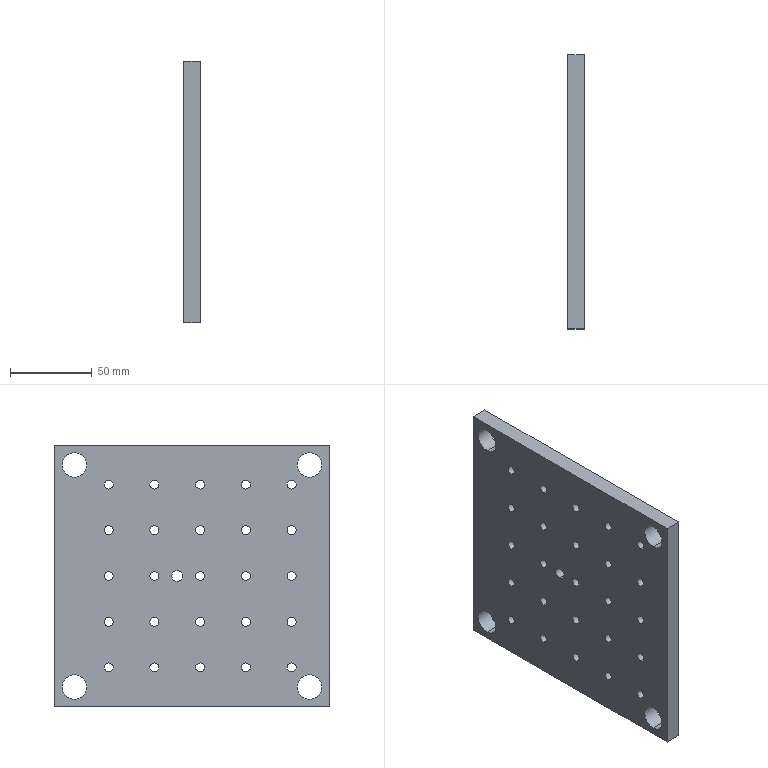Part | STEP file | 03-14 Suction column fixing plate | 1 solid | 141 faces | box 10 x 168 x 160 mm | volume 247896 mm3 | cylinder 110 | plane 31 | commonest cylinder face diameters 5.5 x50 10 x50 15 x8 6.8 x2